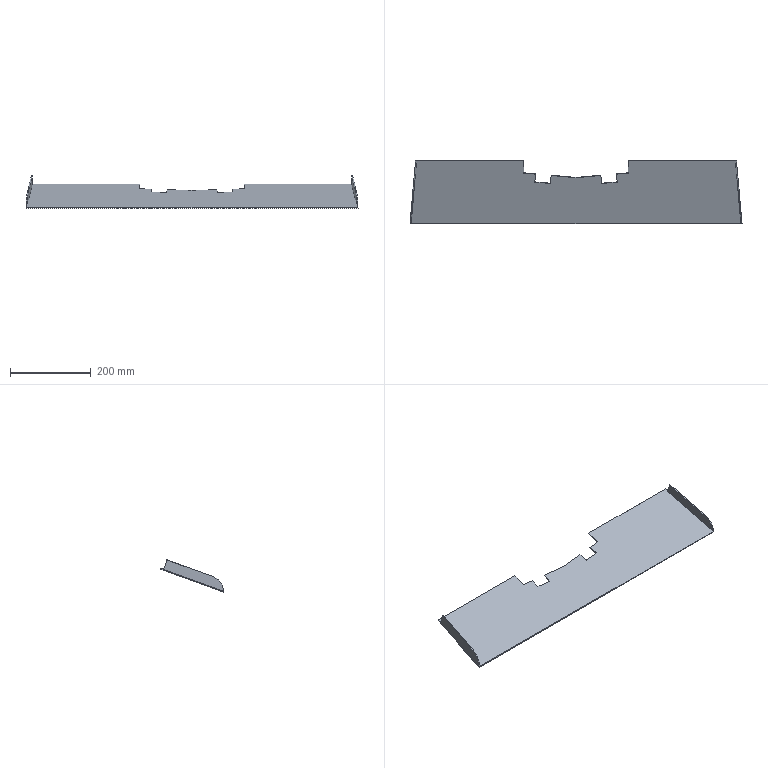Part | NX | features solid 2 | 1 solid | 31 faces | box 824.812 x 157.452 x 80.048 mm | volume 262408 mm3 | plane 27 | spline 2 | cylinder 2 | commonest cylinder face diameters 80 x2
STEP:
#1=CARTESIAN_POINT('',(410.34,-650.,-185.179));
#2=VERTEX_POINT('',#1);
#3=CARTESIAN_POINT('',(-410.34,-650.,-185.179));
#4=VERTEX_POINT('',#3);
#5=CARTESIAN_POINT('',(50.,-650.,-185.179));
#6=DIRECTION('',(-1.,0.,0.));
#7=VECTOR('',#6,1000.);
#8=LINE('',#5,#7);
#9=EDGE_CURVE('',#2,#4,#8,.T.);
#10=ORIENTED_EDGE('',*,*,#9,.F.);
#11=CARTESIAN_POINT('',(397.27,-500.615,-130.808));
#12=VERTEX_POINT('',#11);
#13=CARTESIAN_POINT('',(397.27,-500.615,-130.808));
#14=DIRECTION('',(0.08194,-0.9365,-0.3409));
#15=VECTOR('',#14,1000.);
#16=LINE('',#13,#15);
#17=EDGE_CURVE('',#12,#2,#16,.T.);
#18=ORIENTED_EDGE('',*,*,#17,.F.);
#19=CARTESIAN_POINT('',(399.293,-500.463,-130.752));
#20=VERTEX_POINT('',#19);
#21=CARTESIAN_POINT('',(399.263,-500.461,-130.752));
#22=DIRECTION('',(-0.9966,-0.07699,-0.02802));
#23=VECTOR('',#22,1000.);
#24=LINE('',#21,#23);
#25=EDGE_CURVE('',#20,#12,#24,.T.);
#26=ORIENTED_EDGE('',*,*,#25,.F.);
#27=CARTESIAN_POINT('',(398.691,-493.232,-128.121));
#28=VERTEX_POINT('',#27);
#29=CARTESIAN_POINT('',(395.486,-456.602,-114.788));
#30=DIRECTION('',(0.08194,-0.9365,-0.3409));
#31=VECTOR('',#30,1000.);
#32=LINE('',#29,#31);
#33=EDGE_CURVE('',#28,#20,#32,.T.);
#34=ORIENTED_EDGE('',*,*,#33,.F.);
#35=CARTESIAN_POINT('',(129.932,-493.232,-128.121));
#36=VERTEX_POINT('',#35);
#37=CARTESIAN_POINT('',(-50.,-493.232,-128.121));
#38=DIRECTION('',(1.,0.,0.));
#39=VECTOR('',#38,1000.);
#40=LINE('',#37,#39);
#41=EDGE_CURVE('',#36,#28,#40,.T.);
#42=ORIENTED_EDGE('',*,*,#41,.F.);
#43=CARTESIAN_POINT('',(130.48,-524.313,-139.433));
#44=VERTEX_POINT('',#43);
#45=CARTESIAN_POINT('',(130.48,-524.313,-139.433));
#46=CARTESIAN_POINT('',(130.297,-513.953,-135.662));
#47=CARTESIAN_POINT('',(130.114,-503.593,-131.891));
#48=CARTESIAN_POINT('',(129.932,-493.232,-128.121));
#49=B_SPLINE_CURVE_WITH_KNOTS('',3,(#45,#46,#47,#48),.UNSPECIFIED.,.F.,.F.,(4,4),(0.,1.),.UNSPECIFIED.);
#50=EDGE_CURVE('',#36,#44,#49,.F.);
#51=ORIENTED_EDGE('',*,*,#50,.T.);
#52=CARTESIAN_POINT('',(100.594,-526.928,-140.385));
#53=VERTEX_POINT('',#52);
#54=CARTESIAN_POINT('',(-45.178,-539.681,-145.027));
#55=DIRECTION('',(0.9957,0.08711,0.03171));
#56=VECTOR('',#55,1000.);
#57=LINE('',#54,#56);
#58=EDGE_CURVE('',#53,#44,#57,.T.);
#59=ORIENTED_EDGE('',*,*,#58,.F.);
#60=CARTESIAN_POINT('',(102.337,-546.852,-147.637));
#61=VERTEX_POINT('',#60);
#62=CARTESIAN_POINT('',(96.463,-479.703,-123.196));
#63=DIRECTION('',(0.08194,-0.9365,-0.3409));
#64=VECTOR('',#63,1000.);
#65=LINE('',#62,#64);
#66=EDGE_CURVE('',#61,#53,#65,.F.);
#67=ORIENTED_EDGE('',*,*,#66,.F.);
#68=CARTESIAN_POINT('',(63.601,-550.241,-148.87));
#69=VERTEX_POINT('',#68);
#70=CARTESIAN_POINT('',(150.417,-542.645,-146.105));
#71=DIRECTION('',(-0.9957,-0.08711,-0.03171));
#72=VECTOR('',#71,1000.);
#73=LINE('',#70,#72);
#74=EDGE_CURVE('',#69,#61,#73,.F.);
#75=ORIENTED_EDGE('',*,*,#74,.F.);
#76=CARTESIAN_POINT('',(61.858,-530.317,-141.618));
#77=VERTEX_POINT('',#76);
#78=CARTESIAN_POINT('',(57.692,-482.698,-124.287));
#79=DIRECTION('',(0.08194,-0.9365,-0.3409));
#80=VECTOR('',#79,1000.);
#81=LINE('',#78,#80);
#82=EDGE_CURVE('',#69,#77,#81,.F.);
#83=ORIENTED_EDGE('',*,*,#82,.T.);
#84=CARTESIAN_POINT('',(0.,-535.729,-143.588));
#85=VERTEX_POINT('',#84);
#86=CARTESIAN_POINT('',(-45.178,-539.681,-145.027));
#87=DIRECTION('',(0.9957,0.08711,0.03171));
#88=VECTOR('',#87,1000.);
#89=LINE('',#86,#88);
#90=EDGE_CURVE('',#85,#77,#89,.T.);
#91=ORIENTED_EDGE('',*,*,#90,.F.);
#92=CARTESIAN_POINT('',(-61.858,-530.317,-141.618));
#93=VERTEX_POINT('',#92);
#94=CARTESIAN_POINT('',(45.178,-539.681,-145.027));
#95=DIRECTION('',(-0.9957,0.08711,0.03171));
#96=VECTOR('',#95,1000.);
#97=LINE('',#94,#96);
#98=EDGE_CURVE('',#85,#93,#97,.T.);
#99=ORIENTED_EDGE('',*,*,#98,.T.);
#100=CARTESIAN_POINT('',(-63.601,-550.241,-148.87));
#101=VERTEX_POINT('',#100);
#102=CARTESIAN_POINT('',(-57.692,-482.698,-124.287));
#103=DIRECTION('',(-0.08194,-0.9365,-0.3409));
#104=VECTOR('',#103,1000.);
#105=LINE('',#102,#104);
#106=EDGE_CURVE('',#101,#93,#105,.F.);
#107=ORIENTED_EDGE('',*,*,#106,.F.);
#108=CARTESIAN_POINT('',(-102.337,-546.852,-147.637));
#109=VERTEX_POINT('',#108);
#110=CARTESIAN_POINT('',(-150.417,-542.645,-146.105));
#111=DIRECTION('',(0.9957,-0.08711,-0.03171));
#112=VECTOR('',#111,1000.);
#113=LINE('',#110,#112);
#114=EDGE_CURVE('',#101,#109,#113,.F.);
#115=ORIENTED_EDGE('',*,*,#114,.T.);
#116=CARTESIAN_POINT('',(-100.594,-526.928,-140.385));
#117=VERTEX_POINT('',#116);
#118=CARTESIAN_POINT('',(-96.463,-479.703,-123.196));
#119=DIRECTION('',(-0.08194,-0.9365,-0.3409));
#120=VECTOR('',#119,1000.);
#121=LINE('',#118,#120);
#122=EDGE_CURVE('',#109,#117,#121,.F.);
#123=ORIENTED_EDGE('',*,*,#122,.T.);
#124=CARTESIAN_POINT('',(-130.48,-524.313,-139.433));
#125=VERTEX_POINT('',#124);
#126=CARTESIAN_POINT('',(45.178,-539.681,-145.027));
#127=DIRECTION('',(-0.9957,0.08711,0.03171));
#128=VECTOR('',#127,1000.);
#129=LINE('',#126,#128);
#130=EDGE_CURVE('',#117,#125,#129,.T.);
#131=ORIENTED_EDGE('',*,*,#130,.T.);
#132=CARTESIAN_POINT('',(-129.932,-493.232,-128.121));
#133=VERTEX_POINT('',#132);
#134=CARTESIAN_POINT('',(-130.48,-524.313,-139.433));
#135=CARTESIAN_POINT('',(-130.297,-513.953,-135.662));
#136=CARTESIAN_POINT('',(-130.114,-503.593,-131.891));
#137=CARTESIAN_POINT('',(-129.932,-493.232,-128.121));
#138=B_SPLINE_CURVE_WITH_KNOTS('',3,(#134,#135,#136,#137),.UNSPECIFIED.,.F.,.F.,(4,4),(0.,1.),.UNSPECIFIED.);
#139=EDGE_CURVE('',#133,#125,#138,.F.);
#140=ORIENTED_EDGE('',*,*,#139,.F.);
#141=CARTESIAN_POINT('',(-398.691,-493.232,-128.121));
#142=VERTEX_POINT('',#141);
#143=CARTESIAN_POINT('',(50.,-493.232,-128.121));
#144=DIRECTION('',(-1.,0.,0.));
#145=VECTOR('',#144,1000.);
#146=LINE('',#143,#145);
#147=EDGE_CURVE('',#133,#142,#146,.T.);
#148=ORIENTED_EDGE('',*,*,#147,.T.);
#149=CARTESIAN_POINT('',(-399.293,-500.463,-130.752));
#150=VERTEX_POINT('',#149);
#151=CARTESIAN_POINT('',(-395.486,-456.602,-114.788));
#152=DIRECTION('',(-0.08194,-0.9365,-0.3409));
#153=VECTOR('',#152,1000.);
#154=LINE('',#151,#153);
#155=EDGE_CURVE('',#142,#150,#154,.T.);
#156=ORIENTED_EDGE('',*,*,#155,.T.);
#157=CARTESIAN_POINT('',(-397.27,-500.615,-130.808));
#158=VERTEX_POINT('',#157);
#159=CARTESIAN_POINT('',(-399.263,-500.461,-130.752));
#160=DIRECTION('',(0.9966,-0.07699,-0.02802));
#161=VECTOR('',#160,1000.);
#162=LINE('',#159,#161);
#163=EDGE_CURVE('',#150,#158,#162,.T.);
#164=ORIENTED_EDGE('',*,*,#163,.T.);
#165=CARTESIAN_POINT('',(-397.27,-500.615,-130.808));
#166=DIRECTION('',(-0.08194,-0.9365,-0.3409));
#167=VECTOR('',#166,1000.);
#168=LINE('',#165,#167);
#169=EDGE_CURVE('',#158,#4,#168,.T.);
#170=ORIENTED_EDGE('',*,*,#169,.T.);
#171=EDGE_LOOP('',(#10,#18,#26,#34,#42,#51,#59,#67,#75,#83,#91,#99,#107,#115,#123,#131,#140,#148,#156,#164,#170));
#172=FACE_BOUND('',#171,.T.);
#173=CARTESIAN_POINT('',(50.,-491.018,-127.315));
#174=DIRECTION('',(0.,-0.342,0.9397));
#175=DIRECTION('',(1.,0.,0.));
#176=AXIS2_PLACEMENT_3D('',#173,#174,#175);
#177=PLANE('',#176);
#178=ADVANCED_FACE('',(#172),#177,.T.);
#179=CARTESIAN_POINT('',(0.,-535.045,-145.467));
#180=VERTEX_POINT('',#179);
#181=CARTESIAN_POINT('',(-61.858,-529.633,-143.498));
#182=VERTEX_POINT('',#181);
#183=CARTESIAN_POINT('',(45.178,-538.997,-146.906));
#184=DIRECTION('',(-0.9957,0.08711,0.03171));
#185=VECTOR('',#184,1000.);
#186=LINE('',#183,#185);
#187=EDGE_CURVE('',#180,#182,#186,.T.);
#188=ORIENTED_EDGE('',*,*,#187,.F.);
#189=CARTESIAN_POINT('',(61.858,-529.633,-143.498));
#190=VERTEX_POINT('',#189);
#191=CARTESIAN_POINT('',(-45.178,-538.997,-146.906));
#192=DIRECTION('',(0.9957,0.08711,0.03171));
#193=VECTOR('',#192,1000.);
#194=LINE('',#191,#193);
#195=EDGE_CURVE('',#180,#190,#194,.T.);
#196=ORIENTED_EDGE('',*,*,#195,.T.);
#197=CARTESIAN_POINT('',(63.601,-549.557,-150.749));
#198=VERTEX_POINT('',#197);
#199=CARTESIAN_POINT('',(57.692,-482.014,-126.166));
#200=DIRECTION('',(0.08194,-0.9365,-0.3409));
#201=VECTOR('',#200,1000.);
#202=LINE('',#199,#201);
#203=EDGE_CURVE('',#198,#190,#202,.F.);
#204=ORIENTED_EDGE('',*,*,#203,.F.);
#205=CARTESIAN_POINT('',(102.337,-546.168,-149.516));
#206=VERTEX_POINT('',#205);
#207=CARTESIAN_POINT('',(150.417,-541.961,-147.985));
#208=DIRECTION('',(-0.9957,-0.08711,-0.03171));
#209=VECTOR('',#208,1000.);
#210=LINE('',#207,#209);
#211=EDGE_CURVE('',#198,#206,#210,.F.);
#212=ORIENTED_EDGE('',*,*,#211,.T.);
#213=CARTESIAN_POINT('',(100.594,-526.244,-142.264));
#214=VERTEX_POINT('',#213);
#215=CARTESIAN_POINT('',(96.463,-479.019,-125.076));
#216=DIRECTION('',(0.08194,-0.9365,-0.3409));
#217=VECTOR('',#216,1000.);
#218=LINE('',#215,#217);
#219=EDGE_CURVE('',#206,#214,#218,.F.);
#220=ORIENTED_EDGE('',*,*,#219,.T.);
#221=CARTESIAN_POINT('',(130.48,-523.629,-141.313));
#222=VERTEX_POINT('',#221);
#223=CARTESIAN_POINT('',(-45.178,-538.997,-146.906));
#224=DIRECTION('',(0.9957,0.08711,0.03171));
#225=VECTOR('',#224,1000.);
#226=LINE('',#223,#225);
#227=EDGE_CURVE('',#214,#222,#226,.T.);
#228=ORIENTED_EDGE('',*,*,#227,.T.);
#229=CARTESIAN_POINT('',(129.932,-492.548,-130.));
#230=VERTEX_POINT('',#229);
#231=CARTESIAN_POINT('',(130.48,-523.629,-141.313));
#232=CARTESIAN_POINT('',(130.297,-513.269,-137.542));
#233=CARTESIAN_POINT('',(130.114,-502.909,-133.771));
#234=CARTESIAN_POINT('',(129.932,-492.548,-130.));
#235=B_SPLINE_CURVE_WITH_KNOTS('',3,(#231,#232,#233,#234),.UNSPECIFIED.,.F.,.F.,(4,4),(0.,1.),.UNSPECIFIED.);
#236=EDGE_CURVE('',#230,#222,#235,.F.);
#237=ORIENTED_EDGE('',*,*,#236,.F.);
#238=CARTESIAN_POINT('',(398.631,-492.548,-130.));
#239=VERTEX_POINT('',#238);
#240=CARTESIAN_POINT('',(-50.,-492.548,-130.));
#241=DIRECTION('',(1.,0.,0.));
#242=VECTOR('',#241,1000.);
#243=LINE('',#240,#242);
#244=EDGE_CURVE('',#230,#239,#243,.T.);
#245=ORIENTED_EDGE('',*,*,#244,.T.);
#246=CARTESIAN_POINT('',(399.263,-499.777,-132.631));
#247=VERTEX_POINT('',#246);
#248=CARTESIAN_POINT('',(395.427,-455.923,-116.669));
#249=DIRECTION('',(0.08194,-0.9365,-0.3409));
#250=VECTOR('',#249,1000.);
#251=LINE('',#248,#250);
#252=EDGE_CURVE('',#239,#247,#251,.T.);
#253=ORIENTED_EDGE('',*,*,#252,.T.);
#254=CARTESIAN_POINT('',(412.406,-650.,-187.308));
#255=VERTEX_POINT('',#254);
#256=CARTESIAN_POINT('',(395.427,-455.923,-116.669));
#257=DIRECTION('',(0.08194,-0.9365,-0.3409));
#258=VECTOR('',#257,1000.);
#259=LINE('',#256,#258);
#260=EDGE_CURVE('',#247,#255,#259,.T.);
#261=ORIENTED_EDGE('',*,*,#260,.T.);
#262=CARTESIAN_POINT('',(-412.406,-650.,-187.308));
#263=VERTEX_POINT('',#262);
#264=CARTESIAN_POINT('',(50.,-650.,-187.308));
#265=DIRECTION('',(-1.,0.,0.));
#266=VECTOR('',#265,1000.);
#267=LINE('',#264,#266);
#268=EDGE_CURVE('',#255,#263,#267,.T.);
#269=ORIENTED_EDGE('',*,*,#268,.T.);
#270=CARTESIAN_POINT('',(-399.263,-499.777,-132.631));
#271=VERTEX_POINT('',#270);
#272=CARTESIAN_POINT('',(-395.427,-455.923,-116.669));
#273=DIRECTION('',(-0.08194,-0.9365,-0.3409));
#274=VECTOR('',#273,1000.);
#275=LINE('',#272,#274);
#276=EDGE_CURVE('',#271,#263,#275,.T.);
#277=ORIENTED_EDGE('',*,*,#276,.F.);
#278=CARTESIAN_POINT('',(-398.631,-492.548,-130.));
#279=VERTEX_POINT('',#278);
#280=CARTESIAN_POINT('',(-395.427,-455.923,-116.669));
#281=DIRECTION('',(-0.08194,-0.9365,-0.3409));
#282=VECTOR('',#281,1000.);
#283=LINE('',#280,#282);
#284=EDGE_CURVE('',#279,#271,#283,.T.);
#285=ORIENTED_EDGE('',*,*,#284,.F.);
#286=CARTESIAN_POINT('',(-129.932,-492.548,-130.));
#287=VERTEX_POINT('',#286);
#288=CARTESIAN_POINT('',(50.,-492.548,-130.));
#289=DIRECTION('',(-1.,0.,0.));
#290=VECTOR('',#289,1000.);
#291=LINE('',#288,#290);
#292=EDGE_CURVE('',#287,#279,#291,.T.);
#293=ORIENTED_EDGE('',*,*,#292,.F.);
#294=CARTESIAN_POINT('',(-130.48,-523.629,-141.313));
#295=VERTEX_POINT('',#294);
#296=CARTESIAN_POINT('',(-130.48,-523.629,-141.313));
#297=CARTESIAN_POINT('',(-130.297,-513.269,-137.542));
#298=CARTESIAN_POINT('',(-130.114,-502.909,-133.771));
#299=CARTESIAN_POINT('',(-129.932,-492.548,-130.));
#300=B_SPLINE_CURVE_WITH_KNOTS('',3,(#296,#297,#298,#299),.UNSPECIFIED.,.F.,.F.,(4,4),(0.,1.),.UNSPECIFIED.);
#301=EDGE_CURVE('',#287,#295,#300,.F.);
#302=ORIENTED_EDGE('',*,*,#301,.T.);
#303=CARTESIAN_POINT('',(-100.594,-526.244,-142.264));
#304=VERTEX_POINT('',#303);
#305=CARTESIAN_POINT('',(45.178,-538.997,-146.906));
#306=DIRECTION('',(-0.9957,0.08711,0.03171));
#307=VECTOR('',#306,1000.);
#308=LINE('',#305,#307);
#309=EDGE_CURVE('',#304,#295,#308,.T.);
#310=ORIENTED_EDGE('',*,*,#309,.F.);
#311=CARTESIAN_POINT('',(-102.337,-546.168,-149.516));
#312=VERTEX_POINT('',#311);
#313=CARTESIAN_POINT('',(-96.463,-479.019,-125.076));
#314=DIRECTION('',(-0.08194,-0.9365,-0.3409));
#315=VECTOR('',#314,1000.);
#316=LINE('',#313,#315);
#317=EDGE_CURVE('',#312,#304,#316,.F.);
#318=ORIENTED_EDGE('',*,*,#317,.F.);
#319=CARTESIAN_POINT('',(-63.601,-549.557,-150.749));
#320=VERTEX_POINT('',#319);
#321=CARTESIAN_POINT('',(-150.417,-541.961,-147.985));
#322=DIRECTION('',(0.9957,-0.08711,-0.03171));
#323=VECTOR('',#322,1000.);
#324=LINE('',#321,#323);
#325=EDGE_CURVE('',#320,#312,#324,.F.);
#326=ORIENTED_EDGE('',*,*,#325,.F.);
#327=CARTESIAN_POINT('',(-57.692,-482.014,-126.166));
#328=DIRECTION('',(-0.08194,-0.9365,-0.3409));
#329=VECTOR('',#328,1000.);
#330=LINE('',#327,#329);
#331=EDGE_CURVE('',#320,#182,#330,.F.);
#332=ORIENTED_EDGE('',*,*,#331,.T.);
#333=EDGE_LOOP('',(#188,#196,#204,#212,#220,#228,#237,#245,#253,#261,#269,#277,#285,#293,#302,#310,#318,#326,#332));
#334=FACE_BOUND('',#333,.T.);
#335=CARTESIAN_POINT('',(50.,-490.334,-129.194));
#336=DIRECTION('',(0.,-0.342,0.9397));
#337=DIRECTION('',(1.,0.,0.));
#338=AXIS2_PLACEMENT_3D('',#335,#336,#337);
#339=PLANE('',#338);
#340=ADVANCED_FACE('',(#334),#339,.F.);
#341=ORIENTED_EDGE('',*,*,#268,.F.);
#342=CARTESIAN_POINT('',(412.346,-650.,-185.179));
#343=VERTEX_POINT('',#342);
#344=CARTESIAN_POINT('',(422.793,-650.,-556.706));
#345=DIRECTION('',(0.02811,0.,-0.9996));
#346=VECTOR('',#345,1000.);
#347=LINE('',#344,#346);
#348=EDGE_CURVE('',#343,#255,#347,.T.);
#349=ORIENTED_EDGE('',*,*,#348,.F.);
#350=CARTESIAN_POINT('',(-50.,-650.,-185.179));
#351=DIRECTION('',(1.,0.,0.));
#352=VECTOR('',#351,1000.);
#353=LINE('',#350,#352);
#354=EDGE_CURVE('',#343,#2,#353,.F.);
#355=ORIENTED_EDGE('',*,*,#354,.T.);
#356=ORIENTED_EDGE('',*,*,#9,.T.);
#357=CARTESIAN_POINT('',(-412.346,-650.,-185.179));
#358=VERTEX_POINT('',#357);
#359=CARTESIAN_POINT('',(50.,-650.,-185.179));
#360=DIRECTION('',(-1.,0.,0.));
#361=VECTOR('',#360,1000.);
#362=LINE('',#359,#361);
#363=EDGE_CURVE('',#358,#4,#362,.F.);
#364=ORIENTED_EDGE('',*,*,#363,.F.);
#365=CARTESIAN_POINT('',(-422.793,-650.,-556.706));
#366=DIRECTION('',(-0.02811,0.,-0.9996));
#367=VECTOR('',#366,1000.);
#368=LINE('',#365,#367);
#369=EDGE_CURVE('',#358,#263,#368,.T.);
#370=ORIENTED_EDGE('',*,*,#369,.T.);
#371=EDGE_LOOP('',(#341,#349,#355,#356,#364,#370));
#372=FACE_BOUND('',#371,.T.);
#373=CARTESIAN_POINT('',(50.,-650.,-570.));
#374=DIRECTION('',(0.,1.,0.));
#375=DIRECTION('',(-1.,0.,0.));
#376=AXIS2_PLACEMENT_3D('',#373,#374,#375);
#377=PLANE('',#376);
#378=ADVANCED_FACE('',(#372),#377,.F.);
#379=CARTESIAN_POINT('',(-398.289,-488.644,-140.726));
#380=DIRECTION('',(0.02991,0.3419,-0.9393));
#381=VECTOR('',#380,1000.);
#382=LINE('',#379,#381);
#383=EDGE_CURVE('',#142,#279,#382,.T.);
#384=ORIENTED_EDGE('',*,*,#383,.F.);
#385=ORIENTED_EDGE('',*,*,#147,.F.);
#386=CARTESIAN_POINT('',(-129.932,-493.232,-128.121));
#387=CARTESIAN_POINT('',(-129.932,-493.004,-128.747));
#388=CARTESIAN_POINT('',(-129.932,-492.776,-129.374));
#389=CARTESIAN_POINT('',(-129.932,-492.548,-130.));
#390=B_SPLINE_CURVE_WITH_KNOTS('',3,(#386,#387,#388,#389),.UNSPECIFIED.,.F.,.F.,(4,4),(0.,1.),.UNSPECIFIED.);
#391=EDGE_CURVE('',#133,#287,#390,.T.);
#392=ORIENTED_EDGE('',*,*,#391,.T.);
#393=ORIENTED_EDGE('',*,*,#292,.T.);
#394=EDGE_LOOP('',(#384,#385,#392,#393));
#395=FACE_BOUND('',#394,.T.);
#396=CARTESIAN_POINT('',(50.,-493.232,-128.121));
#397=DIRECTION('',(0.,-0.9397,-0.342));
#398=DIRECTION('',(0.,0.342,-0.9397));
#399=AXIS2_PLACEMENT_3D('',#396,#397,#398);
#400=PLANE('',#399);
#401=ADVANCED_FACE('',(#395),#400,.F.);
#402=CARTESIAN_POINT('',(-399.263,-499.777,-132.631));
#403=CARTESIAN_POINT('',(-399.263,-500.005,-132.005));
#404=CARTESIAN_POINT('',(-399.263,-500.233,-131.378));
#405=CARTESIAN_POINT('',(-399.263,-500.461,-130.752));
#406=B_SPLINE_CURVE_WITH_KNOTS('',3,(#402,#403,#404,#405),.UNSPECIFIED.,.F.,.F.,(4,4),(0.,1.),.UNSPECIFIED.);
#407=EDGE_CURVE('',#150,#271,#406,.F.);
#408=ORIENTED_EDGE('',*,*,#407,.F.);
#409=CARTESIAN_POINT('',(-399.392,-501.247,-128.614));
#410=DIRECTION('',(0.03005,0.3435,-0.9387));
#411=VECTOR('',#410,1000.);
#412=LINE('',#409,#411);
#413=EDGE_CURVE('',#150,#271,#412,.T.);
#414=ORIENTED_EDGE('',*,*,#413,.T.);
#415=EDGE_LOOP('',(#408,#414));
#416=FACE_BOUND('',#415,.T.);
#417=CARTESIAN_POINT('',(-474.901,-504.477,-132.213));
#418=DIRECTION('',(0.05641,-0.9382,-0.3415));
#419=DIRECTION('',(0.,0.342,-0.9397));
#420=AXIS2_PLACEMENT_3D('',#417,#418,#419);
#421=PLANE('',#420);
#422=ADVANCED_FACE('',(#416),#421,.T.);
#423=ORIENTED_EDGE('',*,*,#187,.T.);
#424=CARTESIAN_POINT('',(-61.858,-530.317,-141.618));
#425=DIRECTION('',(0.,0.342,-0.9397));
#426=VECTOR('',#425,1000.);
#427=LINE('',#424,#426);
#428=EDGE_CURVE('',#93,#182,#427,.T.);
#429=ORIENTED_EDGE('',*,*,#428,.F.);
#430=ORIENTED_EDGE('',*,*,#98,.F.);
#431=CARTESIAN_POINT('',(0.,-519.209,-188.977));
#432=DIRECTION('',(0.,0.342,-0.9397));
#433=VECTOR('',#432,1000.);
#434=LINE('',#431,#433);
#435=EDGE_CURVE('',#85,#180,#434,.T.);
#436=ORIENTED_EDGE('',*,*,#435,.T.);
#437=EDGE_LOOP('',(#423,#429,#430,#436));
#438=FACE_BOUND('',#437,.T.);
#439=CARTESIAN_POINT('',(45.178,-539.681,-145.027));
#440=DIRECTION('',(-0.0927,-0.9356,-0.3405));
#441=DIRECTION('',(0.,0.342,-0.9397));
#442=AXIS2_PLACEMENT_3D('',#439,#440,#441);
#443=PLANE('',#442);
#444=ADVANCED_FACE('',(#438),#443,.F.);
#445=ORIENTED_EDGE('',*,*,#331,.F.);
#446=CARTESIAN_POINT('',(-63.601,-550.241,-148.87));
#447=DIRECTION('',(0.,0.342,-0.9397));
#448=VECTOR('',#447,1000.);
#449=LINE('',#446,#448);
#450=EDGE_CURVE('',#101,#320,#449,.T.);
#451=ORIENTED_EDGE('',*,*,#450,.F.);
#452=ORIENTED_EDGE('',*,*,#106,.T.);
#453=ORIENTED_EDGE('',*,*,#428,.T.);
#454=EDGE_LOOP('',(#445,#451,#452,#453));
#455=FACE_BOUND('',#454,.T.);
#456=CARTESIAN_POINT('',(-57.692,-482.698,-124.287));
#457=DIRECTION('',(-0.9966,0.07699,0.02802));
#458=DIRECTION('',(-0.07702,-0.997,0.));
#459=AXIS2_PLACEMENT_3D('',#456,#457,#458);
#460=PLANE('',#459);
#461=ADVANCED_FACE('',(#455),#460,.T.);
#462=ORIENTED_EDGE('',*,*,#325,.T.);
#463=CARTESIAN_POINT('',(-102.337,-546.852,-147.637));
#464=DIRECTION('',(0.,0.342,-0.9397));
#465=VECTOR('',#464,1000.);
#466=LINE('',#463,#465);
#467=EDGE_CURVE('',#109,#312,#466,.T.);
#468=ORIENTED_EDGE('',*,*,#467,.F.);
#469=ORIENTED_EDGE('',*,*,#114,.F.);
#470=ORIENTED_EDGE('',*,*,#450,.T.);
#471=EDGE_LOOP('',(#462,#468,#469,#470));
#472=FACE_BOUND('',#471,.T.);
#473=CARTESIAN_POINT('',(-150.417,-542.645,-146.105));
#474=DIRECTION('',(-0.0927,-0.9356,-0.3405));
#475=DIRECTION('',(0.,0.342,-0.9397));
#476=AXIS2_PLACEMENT_3D('',#473,#474,#475);
#477=PLANE('',#476);
#478=ADVANCED_FACE('',(#472),#477,.F.);
#479=ORIENTED_EDGE('',*,*,#317,.T.);
#480=CARTESIAN_POINT('',(-100.594,-526.928,-140.385));
#481=DIRECTION('',(0.,0.342,-0.9397));
#482=VECTOR('',#481,1000.);
#483=LINE('',#480,#482);
#484=EDGE_CURVE('',#117,#304,#483,.T.);
#485=ORIENTED_EDGE('',*,*,#484,.F.);
#486=ORIENTED_EDGE('',*,*,#122,.F.);
#487=ORIENTED_EDGE('',*,*,#467,.T.);
#488=EDGE_LOOP('',(#479,#485,#486,#487));
#489=FACE_BOUND('',#488,.T.);
#490=CARTESIAN_POINT('',(-96.463,-479.703,-123.196));
#491=DIRECTION('',(-0.9966,0.07699,0.02802));
#492=DIRECTION('',(-0.07702,-0.997,0.));
#493=AXIS2_PLACEMENT_3D('',#490,#491,#492);
#494=PLANE('',#493);
#495=ADVANCED_FACE('',(#489),#494,.F.);
#496=ORIENTED_EDGE('',*,*,#309,.T.);
#497=CARTESIAN_POINT('',(-130.48,-523.629,-141.313));
#498=CARTESIAN_POINT('',(-130.48,-523.857,-140.686));
#499=CARTESIAN_POINT('',(-130.48,-524.085,-140.06));
#500=CARTESIAN_POINT('',(-130.48,-524.313,-139.433));
#501=B_SPLINE_CURVE_WITH_KNOTS('',3,(#497,#498,#499,#500),.UNSPECIFIED.,.F.,.F.,(4,4),(0.,1.),.UNSPECIFIED.);
#502=EDGE_CURVE('',#125,#295,#501,.F.);
#503=ORIENTED_EDGE('',*,*,#502,.F.);
#504=ORIENTED_EDGE('',*,*,#130,.F.);
#505=ORIENTED_EDGE('',*,*,#484,.T.);
#506=EDGE_LOOP('',(#496,#503,#504,#505));
#507=FACE_BOUND('',#506,.T.);
#508=CARTESIAN_POINT('',(45.178,-539.681,-145.027));
#509=DIRECTION('',(-0.0927,-0.9356,-0.3405));
#510=DIRECTION('',(0.,0.342,-0.9397));
#511=AXIS2_PLACEMENT_3D('',#508,#509,#510);
#512=PLANE('',#511);
#513=ADVANCED_FACE('',(#507),#512,.F.);
#514=ORIENTED_EDGE('',*,*,#301,.F.);
#515=ORIENTED_EDGE('',*,*,#391,.F.);
#516=ORIENTED_EDGE('',*,*,#139,.T.);
#517=ORIENTED_EDGE('',*,*,#502,.T.);
#518=EDGE_LOOP('',(#514,#515,#516,#517));
#519=FACE_BOUND('',#518,.T.);
#520=CARTESIAN_POINT('',(-130.48,-524.313,-139.433));
#521=DIRECTION('',(0.9999,-0.01558,-0.00567));
#522=DIRECTION('',(0.01558,0.9999,0.));
#523=AXIS2_PLACEMENT_3D('',#520,#521,#522);
#524=PLANE('',#523);
#525=ADVANCED_FACE('',(#519),#524,.T.);
#526=ORIENTED_EDGE('',*,*,#276,.T.);
#527=ORIENTED_EDGE('',*,*,#369,.F.);
#528=CARTESIAN_POINT('',(-409.298,-623.706,-149.005));
#529=VERTEX_POINT('',#528);
#530=CARTESIAN_POINT('',(-409.298,-610.025,-186.592));
#531=DIRECTION('',(-0.9966,0.07699,0.02802));
#532=DIRECTION('',(-0.08194,-0.9365,-0.3409));
#533=AXIS2_PLACEMENT_3D('',#530,#531,#532);
#534=ELLIPSE('',#533,40.135,40.);
#535=EDGE_CURVE('',#358,#529,#534,.T.);
#536=ORIENTED_EDGE('',*,*,#535,.T.);
#537=CARTESIAN_POINT('',(-399.263,-509.012,-107.259));
#538=VERTEX_POINT('',#537);
#539=CARTESIAN_POINT('',(-399.263,-509.012,-107.259));
#540=DIRECTION('',(-0.08194,-0.9365,-0.3409));
#541=VECTOR('',#540,1000.);
#542=LINE('',#539,#541);
#543=EDGE_CURVE('',#538,#529,#542,.T.);
#544=ORIENTED_EDGE('',*,*,#543,.F.);
#545=CARTESIAN_POINT('',(-399.263,-500.461,-130.752));
#546=DIRECTION('',(0.,-0.342,0.9397));
#547=VECTOR('',#546,1000.);
#548=LINE('',#545,#547);
#549=EDGE_CURVE('',#150,#538,#548,.T.);
#550=ORIENTED_EDGE('',*,*,#549,.F.);
#551=ORIENTED_EDGE('',*,*,#407,.T.);
#552=EDGE_LOOP('',(#526,#527,#536,#544,#550,#551));
#553=FACE_BOUND('',#552,.T.);
#554=CARTESIAN_POINT('',(-395.427,-456.607,-114.79));
#555=DIRECTION('',(0.9966,-0.07699,-0.02802));
#556=DIRECTION('',(0.07702,0.997,0.));
#557=AXIS2_PLACEMENT_3D('',#554,#555,#556);
#558=PLANE('',#557);
#559=ADVANCED_FACE('',(#553),#558,.F.);
#560=ORIENTED_EDGE('',*,*,#155,.F.);
#561=ORIENTED_EDGE('',*,*,#383,.T.);
#562=ORIENTED_EDGE('',*,*,#284,.T.);
#563=ORIENTED_EDGE('',*,*,#413,.F.);
#564=EDGE_LOOP('',(#560,#561,#562,#563));
#565=FACE_BOUND('',#564,.T.);
#566=CARTESIAN_POINT('',(-398.627,-492.501,-132.658));
#567=CARTESIAN_POINT('',(-398.627,-492.501,-128.094));
#568=CARTESIAN_POINT('',(-399.328,-500.512,-132.658));
#569=CARTESIAN_POINT('',(-399.328,-500.512,-128.094));
#570=B_SPLINE_SURFACE_WITH_KNOTS('',1,1,((#566,#567),(#568,#569)),.PLANE_SURF.,.F.,.F.,.F.,(2,2),(2,2),(0.3132,0.3354),(0.4939,0.5104),.PIECEWISE_BEZIER_KNOTS.);
#571=ADVANCED_FACE('',(#565),#570,.T.);
#572=ORIENTED_EDGE('',*,*,#163,.F.);
#573=ORIENTED_EDGE('',*,*,#549,.T.);
#574=CARTESIAN_POINT('',(-397.27,-509.166,-107.315));
#575=VERTEX_POINT('',#574);
#576=CARTESIAN_POINT('',(-399.263,-509.012,-107.259));
#577=DIRECTION('',(0.9966,-0.07699,-0.02802));
#578=VECTOR('',#577,1000.);
#579=LINE('',#576,#578);
#580=EDGE_CURVE('',#538,#575,#579,.T.);
#581=ORIENTED_EDGE('',*,*,#580,.T.);
#582=CARTESIAN_POINT('',(-397.27,-500.615,-130.808));
#583=DIRECTION('',(0.,-0.342,0.9397));
#584=VECTOR('',#583,1000.);
#585=LINE('',#582,#584);
#586=EDGE_CURVE('',#158,#575,#585,.T.);
#587=ORIENTED_EDGE('',*,*,#586,.F.);
#588=EDGE_LOOP('',(#572,#573,#581,#587));
#589=FACE_BOUND('',#588,.T.);
#590=CARTESIAN_POINT('',(-399.263,-500.461,-130.752));
#591=DIRECTION('',(-0.08194,-0.9365,-0.3409));
#592=DIRECTION('',(0.,-0.342,0.9397));
#593=AXIS2_PLACEMENT_3D('',#590,#591,#592);
#594=PLANE('',#593);
#595=ADVANCED_FACE('',(#589),#594,.F.);
#596=ORIENTED_EDGE('',*,*,#543,.T.);
#597=CARTESIAN_POINT('',(-407.291,-623.706,-149.005));
#598=VERTEX_POINT('',#597);
#599=CARTESIAN_POINT('',(-409.592,-623.706,-149.005));
#600=DIRECTION('',(-1.,0.,0.));
#601=VECTOR('',#600,1000.);
#602=LINE('',#599,#601);
#603=EDGE_CURVE('',#529,#598,#602,.F.);
#604=ORIENTED_EDGE('',*,*,#603,.T.);
#605=CARTESIAN_POINT('',(-397.27,-509.166,-107.315));
#606=DIRECTION('',(-0.08194,-0.9365,-0.3409));
#607=VECTOR('',#606,1000.);
#608=LINE('',#605,#607);
#609=EDGE_CURVE('',#575,#598,#608,.T.);
#610=ORIENTED_EDGE('',*,*,#609,.F.);
#611=ORIENTED_EDGE('',*,*,#580,.F.);
#612=EDGE_LOOP('',(#596,#604,#610,#611));
#613=FACE_BOUND('',#612,.T.);
#614=CARTESIAN_POINT('',(-399.263,-509.012,-107.259));
#615=DIRECTION('',(0.,0.342,-0.9397));
#616=DIRECTION('',(-0.08194,-0.9365,-0.3409));
#617=AXIS2_PLACEMENT_3D('',#614,#615,#616);
#618=PLANE('',#617);
#619=ADVANCED_FACE('',(#613),#618,.F.);
#620=ORIENTED_EDGE('',*,*,#609,.T.);
#621=CARTESIAN_POINT('',(-407.291,-610.025,-186.592));
#622=DIRECTION('',(-0.9966,0.07699,0.02802));
#623=DIRECTION('',(-0.08194,-0.9365,-0.3409));
#624=AXIS2_PLACEMENT_3D('',#621,#622,#623);
#625=ELLIPSE('',#624,40.135,40.);
#626=EDGE_CURVE('',#598,#4,#625,.F.);
#627=ORIENTED_EDGE('',*,*,#626,.T.);
#628=ORIENTED_EDGE('',*,*,#169,.F.);
#629=ORIENTED_EDGE('',*,*,#586,.T.);
#630=EDGE_LOOP('',(#620,#627,#628,#629));
#631=FACE_BOUND('',#630,.T.);
#632=CARTESIAN_POINT('',(-397.27,-500.615,-130.808));
#633=DIRECTION('',(-0.9966,0.07699,0.02802));
#634=DIRECTION('',(-0.07702,-0.997,0.));
#635=AXIS2_PLACEMENT_3D('',#632,#633,#634);
#636=PLANE('',#635);
#637=ADVANCED_FACE('',(#631),#636,.F.);
#638=ORIENTED_EDGE('',*,*,#535,.F.);
#639=ORIENTED_EDGE('',*,*,#363,.T.);
#640=ORIENTED_EDGE('',*,*,#626,.F.);
#641=ORIENTED_EDGE('',*,*,#603,.F.);
#642=EDGE_LOOP('',(#638,#639,#640,#641));
#643=FACE_BOUND('',#642,.T.);
#644=CARTESIAN_POINT('',(50.,-610.025,-186.592));
#645=DIRECTION('',(-1.,0.,0.));
#646=DIRECTION('',(0.,0.,1.));
#647=AXIS2_PLACEMENT_3D('',#644,#645,#646);
#648=CYLINDRICAL_SURFACE('',#647,40.);
#649=ADVANCED_FACE('',(#643),#648,.T.);
#650=CARTESIAN_POINT('',(398.289,-488.644,-140.726));
#651=DIRECTION('',(-0.02991,0.3419,-0.9393));
#652=VECTOR('',#651,1000.);
#653=LINE('',#650,#652);
#654=EDGE_CURVE('',#28,#239,#653,.T.);
#655=ORIENTED_EDGE('',*,*,#654,.T.);
#656=ORIENTED_EDGE('',*,*,#244,.F.);
#657=CARTESIAN_POINT('',(129.932,-493.232,-128.121));
#658=CARTESIAN_POINT('',(129.932,-493.004,-128.747));
#659=CARTESIAN_POINT('',(129.932,-492.776,-129.374));
#660=CARTESIAN_POINT('',(129.932,-492.548,-130.));
#661=B_SPLINE_CURVE_WITH_KNOTS('',3,(#657,#658,#659,#660),.UNSPECIFIED.,.F.,.F.,(4,4),(0.,1.),.UNSPECIFIED.);
#662=EDGE_CURVE('',#36,#230,#661,.T.);
#663=ORIENTED_EDGE('',*,*,#662,.F.);
#664=ORIENTED_EDGE('',*,*,#41,.T.);
#665=EDGE_LOOP('',(#655,#656,#663,#664));
#666=FACE_BOUND('',#665,.T.);
#667=CARTESIAN_POINT('',(-50.,-493.232,-128.121));
#668=DIRECTION('',(0.,-0.9397,-0.342));
#669=DIRECTION('',(0.,0.342,-0.9397));
#670=AXIS2_PLACEMENT_3D('',#667,#668,#669);
#671=PLANE('',#670);
#672=ADVANCED_FACE('',(#666),#671,.F.);
#673=CARTESIAN_POINT('',(399.263,-499.777,-132.631));
#674=CARTESIAN_POINT('',(399.263,-500.005,-132.005));
#675=CARTESIAN_POINT('',(399.263,-500.233,-131.378));
#676=CARTESIAN_POINT('',(399.263,-500.461,-130.752));
#677=B_SPLINE_CURVE_WITH_KNOTS('',3,(#673,#674,#675,#676),.UNSPECIFIED.,.F.,.F.,(4,4),(0.,1.),.UNSPECIFIED.);
#678=EDGE_CURVE('',#20,#247,#677,.F.);
#679=ORIENTED_EDGE('',*,*,#678,.T.);
#680=CARTESIAN_POINT('',(399.392,-501.247,-128.614));
#681=DIRECTION('',(-0.03005,0.3435,-0.9387));
#682=VECTOR('',#681,1000.);
#683=LINE('',#680,#682);
#684=EDGE_CURVE('',#20,#247,#683,.T.);
#685=ORIENTED_EDGE('',*,*,#684,.F.);
#686=EDGE_LOOP('',(#679,#685));
#687=FACE_BOUND('',#686,.T.);
#688=CARTESIAN_POINT('',(474.901,-504.477,-132.213));
#689=DIRECTION('',(-0.05641,-0.9382,-0.3415));
#690=DIRECTION('',(0.,0.342,-0.9397));
#691=AXIS2_PLACEMENT_3D('',#688,#689,#690);
#692=PLANE('',#691);
#693=ADVANCED_FACE('',(#687),#692,.T.);
#694=ORIENTED_EDGE('',*,*,#195,.F.);
#695=ORIENTED_EDGE('',*,*,#435,.F.);
#696=ORIENTED_EDGE('',*,*,#90,.T.);
#697=CARTESIAN_POINT('',(61.858,-530.317,-141.618));
#698=DIRECTION('',(0.,0.342,-0.9397));
#699=VECTOR('',#698,1000.);
#700=LINE('',#697,#699);
#701=EDGE_CURVE('',#77,#190,#700,.T.);
#702=ORIENTED_EDGE('',*,*,#701,.T.);
#703=EDGE_LOOP('',(#694,#695,#696,#702));
#704=FACE_BOUND('',#703,.T.);
#705=CARTESIAN_POINT('',(-45.178,-539.681,-145.027));
#706=DIRECTION('',(0.0927,-0.9356,-0.3405));
#707=DIRECTION('',(0.,0.342,-0.9397));
#708=AXIS2_PLACEMENT_3D('',#705,#706,#707);
#709=PLANE('',#708);
#710=ADVANCED_FACE('',(#704),#709,.F.);
#711=ORIENTED_EDGE('',*,*,#203,.T.);
#712=ORIENTED_EDGE('',*,*,#701,.F.);
#713=ORIENTED_EDGE('',*,*,#82,.F.);
#714=CARTESIAN_POINT('',(63.601,-550.241,-148.87));
#715=DIRECTION('',(0.,0.342,-0.9397));
#716=VECTOR('',#715,1000.);
#717=LINE('',#714,#716);
#718=EDGE_CURVE('',#69,#198,#717,.T.);
#719=ORIENTED_EDGE('',*,*,#718,.T.);
#720=EDGE_LOOP('',(#711,#712,#713,#719));
#721=FACE_BOUND('',#720,.T.);
#722=CARTESIAN_POINT('',(57.692,-482.698,-124.287));
#723=DIRECTION('',(0.9966,0.07699,0.02802));
#724=DIRECTION('',(0.07702,-0.997,0.));
#725=AXIS2_PLACEMENT_3D('',#722,#723,#724);
#726=PLANE('',#725);
#727=ADVANCED_FACE('',(#721),#726,.T.);
#728=ORIENTED_EDGE('',*,*,#211,.F.);
#729=ORIENTED_EDGE('',*,*,#718,.F.);
#730=ORIENTED_EDGE('',*,*,#74,.T.);
#731=CARTESIAN_POINT('',(102.337,-546.852,-147.637));
#732=DIRECTION('',(0.,0.342,-0.9397));
#733=VECTOR('',#732,1000.);
#734=LINE('',#731,#733);
#735=EDGE_CURVE('',#61,#206,#734,.T.);
#736=ORIENTED_EDGE('',*,*,#735,.T.);
#737=EDGE_LOOP('',(#728,#729,#730,#736));
#738=FACE_BOUND('',#737,.T.);
#739=CARTESIAN_POINT('',(150.417,-542.645,-146.105));
#740=DIRECTION('',(0.0927,-0.9356,-0.3405));
#741=DIRECTION('',(0.,0.342,-0.9397));
#742=AXIS2_PLACEMENT_3D('',#739,#740,#741);
#743=PLANE('',#742);
#744=ADVANCED_FACE('',(#738),#743,.F.);
#745=ORIENTED_EDGE('',*,*,#219,.F.);
#746=ORIENTED_EDGE('',*,*,#735,.F.);
#747=ORIENTED_EDGE('',*,*,#66,.T.);
#748=CARTESIAN_POINT('',(100.594,-526.928,-140.385));
#749=DIRECTION('',(0.,0.342,-0.9397));
#750=VECTOR('',#749,1000.);
#751=LINE('',#748,#750);
#752=EDGE_CURVE('',#53,#214,#751,.T.);
#753=ORIENTED_EDGE('',*,*,#752,.T.);
#754=EDGE_LOOP('',(#745,#746,#747,#753));
#755=FACE_BOUND('',#754,.T.);
#756=CARTESIAN_POINT('',(96.463,-479.703,-123.196));
#757=DIRECTION('',(0.9966,0.07699,0.02802));
#758=DIRECTION('',(0.07702,-0.997,0.));
#759=AXIS2_PLACEMENT_3D('',#756,#757,#758);
#760=PLANE('',#759);
#761=ADVANCED_FACE('',(#755),#760,.F.);
#762=ORIENTED_EDGE('',*,*,#227,.F.);
#763=ORIENTED_EDGE('',*,*,#752,.F.);
#764=ORIENTED_EDGE('',*,*,#58,.T.);
#765=CARTESIAN_POINT('',(130.48,-523.629,-141.313));
#766=CARTESIAN_POINT('',(130.48,-523.857,-140.686));
#767=CARTESIAN_POINT('',(130.48,-524.085,-140.06));
#768=CARTESIAN_POINT('',(130.48,-524.313,-139.433));
#769=B_SPLINE_CURVE_WITH_KNOTS('',3,(#765,#766,#767,#768),.UNSPECIFIED.,.F.,.F.,(4,4),(0.,1.),.UNSPECIFIED.);
#770=EDGE_CURVE('',#44,#222,#769,.F.);
#771=ORIENTED_EDGE('',*,*,#770,.T.);
#772=EDGE_LOOP('',(#762,#763,#764,#771));
#773=FACE_BOUND('',#772,.T.);
#774=CARTESIAN_POINT('',(-45.178,-539.681,-145.027));
#775=DIRECTION('',(0.0927,-0.9356,-0.3405));
#776=DIRECTION('',(0.,0.342,-0.9397));
#777=AXIS2_PLACEMENT_3D('',#774,#775,#776);
#778=PLANE('',#777);
#779=ADVANCED_FACE('',(#773),#778,.F.);
#780=ORIENTED_EDGE('',*,*,#236,.T.);
#781=ORIENTED_EDGE('',*,*,#770,.F.);
#782=ORIENTED_EDGE('',*,*,#50,.F.);
#783=ORIENTED_EDGE('',*,*,#662,.T.);
#784=EDGE_LOOP('',(#780,#781,#782,#783));
#785=FACE_BOUND('',#784,.T.);
#786=CARTESIAN_POINT('',(130.48,-524.313,-139.433));
#787=DIRECTION('',(-0.9999,-0.01558,-0.00567));
#788=DIRECTION('',(-0.01558,0.9999,0.));
#789=AXIS2_PLACEMENT_3D('',#786,#787,#788);
#790=PLANE('',#789);
#791=ADVANCED_FACE('',(#785),#790,.T.);
#792=ORIENTED_EDGE('',*,*,#260,.F.);
#793=ORIENTED_EDGE('',*,*,#678,.F.);
#794=CARTESIAN_POINT('',(399.263,-509.012,-107.259));
#795=VERTEX_POINT('',#794);
#796=CARTESIAN_POINT('',(399.263,-500.461,-130.752));
#797=DIRECTION('',(0.,-0.342,0.9397));
#798=VECTOR('',#797,1000.);
#799=LINE('',#796,#798);
#800=EDGE_CURVE('',#20,#795,#799,.T.);
#801=ORIENTED_EDGE('',*,*,#800,.T.);
#802=CARTESIAN_POINT('',(409.298,-623.706,-149.005));
#803=VERTEX_POINT('',#802);
#804=CARTESIAN_POINT('',(399.263,-509.012,-107.259));
#805=DIRECTION('',(0.08194,-0.9365,-0.3409));
#806=VECTOR('',#805,1000.);
#807=LINE('',#804,#806);
#808=EDGE_CURVE('',#795,#803,#807,.T.);
#809=ORIENTED_EDGE('',*,*,#808,.T.);
#810=CARTESIAN_POINT('',(409.298,-610.025,-186.592));
#811=DIRECTION('',(-0.9966,-0.07699,-0.02802));
#812=DIRECTION('',(0.08194,-0.9365,-0.3409));
#813=AXIS2_PLACEMENT_3D('',#810,#811,#812);
#814=ELLIPSE('',#813,40.135,40.);
#815=EDGE_CURVE('',#343,#803,#814,.T.);
#816=ORIENTED_EDGE('',*,*,#815,.F.);
#817=ORIENTED_EDGE('',*,*,#348,.T.);
#818=EDGE_LOOP('',(#792,#793,#801,#809,#816,#817));
#819=FACE_BOUND('',#818,.T.);
#820=CARTESIAN_POINT('',(395.427,-456.607,-114.79));
#821=DIRECTION('',(-0.9966,-0.07699,-0.02802));
#822=DIRECTION('',(-0.07702,0.997,0.));
#823=AXIS2_PLACEMENT_3D('',#820,#821,#822);
#824=PLANE('',#823);
#825=ADVANCED_FACE('',(#819),#824,.F.);
#826=ORIENTED_EDGE('',*,*,#33,.T.);
#827=ORIENTED_EDGE('',*,*,#684,.T.);
#828=ORIENTED_EDGE('',*,*,#252,.F.);
#829=ORIENTED_EDGE('',*,*,#654,.F.);
#830=EDGE_LOOP('',(#826,#827,#828,#829));
#831=FACE_BOUND('',#830,.T.);
#832=CARTESIAN_POINT('',(398.627,-492.501,-132.658));
#833=CARTESIAN_POINT('',(398.627,-492.501,-128.094));
#834=CARTESIAN_POINT('',(399.328,-500.512,-132.658));
#835=CARTESIAN_POINT('',(399.328,-500.512,-128.094));
#836=B_SPLINE_SURFACE_WITH_KNOTS('',1,1,((#832,#833),(#834,#835)),.PLANE_SURF.,.F.,.F.,.F.,(2,2),(2,2),(0.3132,0.3354),(0.4939,0.5104),.PIECEWISE_BEZIER_KNOTS.);
#837=ADVANCED_FACE('',(#831),#836,.F.);
#838=ORIENTED_EDGE('',*,*,#25,.T.);
#839=CARTESIAN_POINT('',(397.27,-509.166,-107.315));
#840=VERTEX_POINT('',#839);
#841=CARTESIAN_POINT('',(397.27,-500.615,-130.808));
#842=DIRECTION('',(0.,-0.342,0.9397));
#843=VECTOR('',#842,1000.);
#844=LINE('',#841,#843);
#845=EDGE_CURVE('',#12,#840,#844,.T.);
#846=ORIENTED_EDGE('',*,*,#845,.T.);
#847=CARTESIAN_POINT('',(399.263,-509.012,-107.259));
#848=DIRECTION('',(-0.9966,-0.07699,-0.02802));
#849=VECTOR('',#848,1000.);
#850=LINE('',#847,#849);
#851=EDGE_CURVE('',#795,#840,#850,.T.);
#852=ORIENTED_EDGE('',*,*,#851,.F.);
#853=ORIENTED_EDGE('',*,*,#800,.F.);
#854=EDGE_LOOP('',(#838,#846,#852,#853));
#855=FACE_BOUND('',#854,.T.);
#856=CARTESIAN_POINT('',(399.263,-500.461,-130.752));
#857=DIRECTION('',(0.08194,-0.9365,-0.3409));
#858=DIRECTION('',(0.,-0.342,0.9397));
#859=AXIS2_PLACEMENT_3D('',#856,#857,#858);
#860=PLANE('',#859);
#861=ADVANCED_FACE('',(#855),#860,.F.);
#862=ORIENTED_EDGE('',*,*,#808,.F.);
#863=ORIENTED_EDGE('',*,*,#851,.T.);
#864=CARTESIAN_POINT('',(407.291,-623.706,-149.005));
#865=VERTEX_POINT('',#864);
#866=CARTESIAN_POINT('',(397.27,-509.166,-107.315));
#867=DIRECTION('',(0.08194,-0.9365,-0.3409));
#868=VECTOR('',#867,1000.);
#869=LINE('',#866,#868);
#870=EDGE_CURVE('',#840,#865,#869,.T.);
#871=ORIENTED_EDGE('',*,*,#870,.T.);
#872=CARTESIAN_POINT('',(409.592,-623.706,-149.005));
#873=DIRECTION('',(1.,0.,0.));
#874=VECTOR('',#873,1000.);
#875=LINE('',#872,#874);
#876=EDGE_CURVE('',#803,#865,#875,.F.);
#877=ORIENTED_EDGE('',*,*,#876,.F.);
#878=EDGE_LOOP('',(#862,#863,#871,#877));
#879=FACE_BOUND('',#878,.T.);
#880=CARTESIAN_POINT('',(399.263,-509.012,-107.259));
#881=DIRECTION('',(0.,0.342,-0.9397));
#882=DIRECTION('',(0.08194,-0.9365,-0.3409));
#883=AXIS2_PLACEMENT_3D('',#880,#881,#882);
#884=PLANE('',#883);
#885=ADVANCED_FACE('',(#879),#884,.F.);
#886=ORIENTED_EDGE('',*,*,#870,.F.);
#887=ORIENTED_EDGE('',*,*,#845,.F.);
#888=ORIENTED_EDGE('',*,*,#17,.T.);
#889=CARTESIAN_POINT('',(407.291,-610.025,-186.592));
#890=DIRECTION('',(-0.9966,-0.07699,-0.02802));
#891=DIRECTION('',(0.08194,-0.9365,-0.3409));
#892=AXIS2_PLACEMENT_3D('',#889,#890,#891);
#893=ELLIPSE('',#892,40.135,40.);
#894=EDGE_CURVE('',#865,#2,#893,.F.);
#895=ORIENTED_EDGE('',*,*,#894,.F.);
#896=EDGE_LOOP('',(#886,#887,#888,#895));
#897=FACE_BOUND('',#896,.T.);
#898=CARTESIAN_POINT('',(397.27,-500.615,-130.808));
#899=DIRECTION('',(0.9966,0.07699,0.02802));
#900=DIRECTION('',(0.07702,-0.997,0.));
#901=AXIS2_PLACEMENT_3D('',#898,#899,#900);
#902=PLANE('',#901);
#903=ADVANCED_FACE('',(#897),#902,.F.);
#904=ORIENTED_EDGE('',*,*,#815,.T.);
#905=ORIENTED_EDGE('',*,*,#876,.T.);
#906=ORIENTED_EDGE('',*,*,#894,.T.);
#907=ORIENTED_EDGE('',*,*,#354,.F.);
#908=EDGE_LOOP('',(#904,#905,#906,#907));
#909=FACE_BOUND('',#908,.T.);
#910=CARTESIAN_POINT('',(-50.,-610.025,-186.592));
#911=DIRECTION('',(1.,0.,0.));
#912=DIRECTION('',(0.,0.,1.));
#913=AXIS2_PLACEMENT_3D('',#910,#911,#912);
#914=CYLINDRICAL_SURFACE('',#913,40.);
#915=ADVANCED_FACE('',(#909),#914,.T.);
#916=CLOSED_SHELL('',(#178,#340,#378,#401,#422,#444,#461,#478,#495,#513,#525,#559,#571,#595,#619,#637,#649,#672,#693,#710,#727,#744,#761,#779,#791,#825,#837,#861,#885,#903,#915));
#917=MANIFOLD_SOLID_BREP('',#916);
#918=(LENGTH_UNIT()NAMED_UNIT(*)SI_UNIT(.MILLI.,.METRE.));
#919=UNCERTAINTY_MEASURE_WITH_UNIT(LENGTH_MEASURE(0.111),#918,'','');
#920=(NAMED_UNIT(*)PLANE_ANGLE_UNIT()SI_UNIT($,.RADIAN.));
#921=(NAMED_UNIT(*)SI_UNIT($,.STERADIAN.)SOLID_ANGLE_UNIT());
#922=(GEOMETRIC_REPRESENTATION_CONTEXT(3)GLOBAL_UNCERTAINTY_ASSIGNED_CONTEXT((#919))GLOBAL_UNIT_ASSIGNED_CONTEXT((#918,#920,#921))REPRESENTATION_CONTEXT('',''));
#923=ADVANCED_BREP_SHAPE_REPRESENTATION('',(#917),#922);